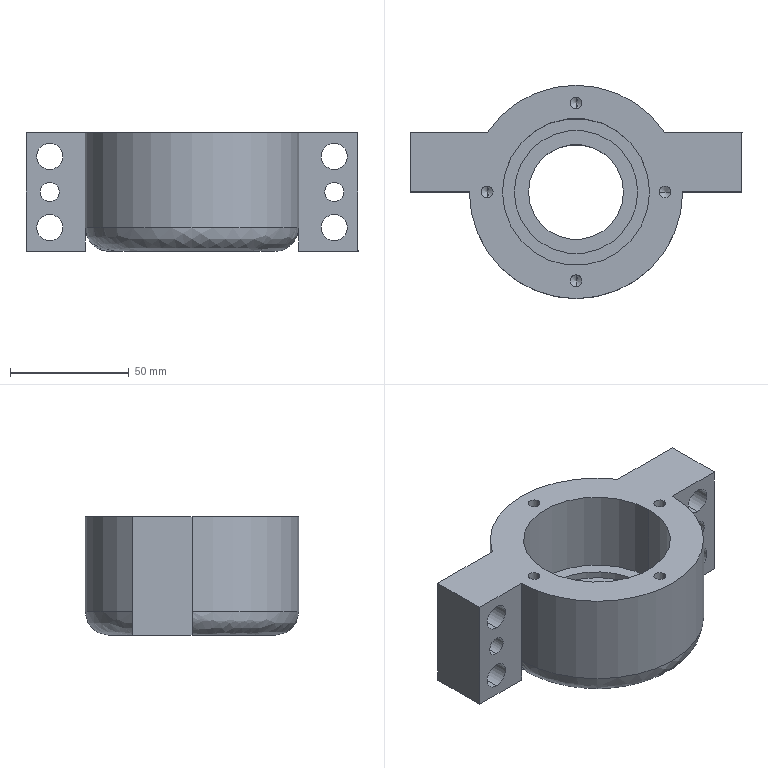Part | STEP file | 45L X Bearing Seat | 1 solid | 69 faces | box 140 x 90 x 50 mm | volume 231952 mm3 | cylinder 38 | plane 21 | cone 8 | spline 2 | commonest cylinder face diameters 5 x8 11 x8 16 x8 8 x4 52 x4 40 x2